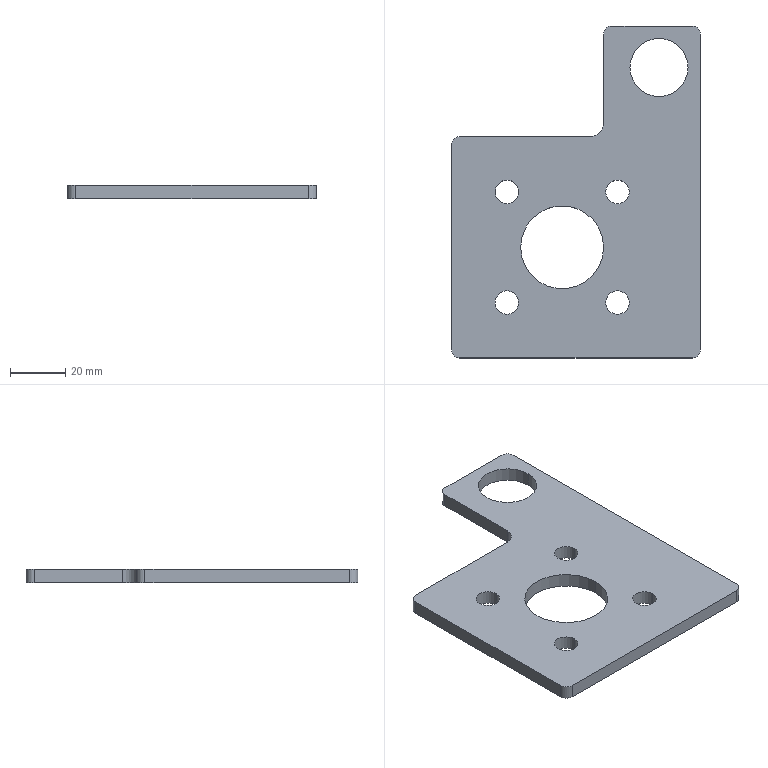Part | STEP file | PN_0060 | 1 solid | 26 faces | box 90 x 120 x 5 mm | volume 36578 mm3 | cylinder 18 | plane 8 | commonest cylinder face diameters 8.5 x8 6 x5 21 x2 30 x2 10 x1